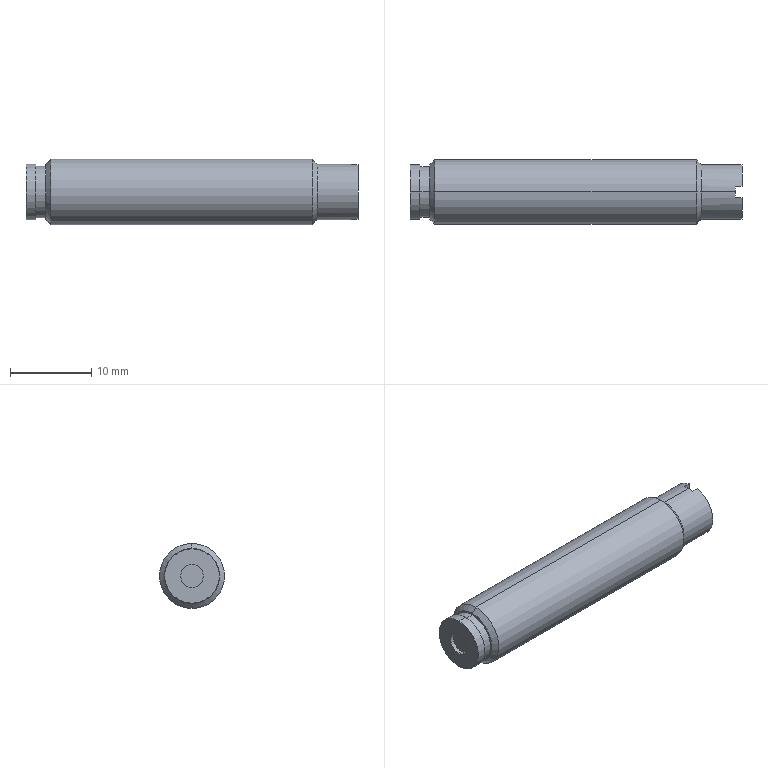Part | SolidWorks | features BaseBody 1 | 1 solid | 26 faces | box 40.8 x 8 x 8 mm | volume 1922 mm3 | cylinder 10 | plane 10 | cone 4 | torus 2 | commonest cylinder face diameters 6.8 x4 2.8 x2 6.3 x2 8 x2
STEP:
#1=CARTESIAN_POINT('',(0.5,0.,1.4));
#2=VERTEX_POINT('',#1);
#3=CARTESIAN_POINT('',(0.5,0.,-1.4));
#4=VERTEX_POINT('',#3);
#5=CARTESIAN_POINT('',(0.5,0.,0.));
#6=DIRECTION('',(1.,0.,0.));
#7=DIRECTION('',(0.,0.,-1.));
#8=AXIS2_PLACEMENT_3D('',#5,#6,#7);
#9=CIRCLE('',#8,1.4);
#10=EDGE_CURVE('',#2,#4,#9,.T.);
#11=ORIENTED_EDGE('',*,*,#10,.T.);
#12=CARTESIAN_POINT('',(0.,0.,-1.4));
#13=VERTEX_POINT('',#12);
#14=CARTESIAN_POINT('',(0.5,0.,-1.4));
#15=DIRECTION('',(-1.,0.,0.));
#16=VECTOR('',#15,1000.);
#17=LINE('',#14,#16);
#18=EDGE_CURVE('',#4,#13,#17,.T.);
#19=ORIENTED_EDGE('',*,*,#18,.T.);
#20=CARTESIAN_POINT('',(0.,0.,1.4));
#21=VERTEX_POINT('',#20);
#22=CARTESIAN_POINT('',(0.,0.,0.));
#23=DIRECTION('',(1.,0.,0.));
#24=DIRECTION('',(0.,0.,-1.));
#25=AXIS2_PLACEMENT_3D('',#22,#23,#24);
#26=CIRCLE('',#25,1.4);
#27=EDGE_CURVE('',#21,#13,#26,.T.);
#28=ORIENTED_EDGE('',*,*,#27,.F.);
#29=CARTESIAN_POINT('',(0.5,0.,1.4));
#30=DIRECTION('',(-1.,0.,0.));
#31=VECTOR('',#30,1000.);
#32=LINE('',#29,#31);
#33=EDGE_CURVE('',#2,#21,#32,.T.);
#34=ORIENTED_EDGE('',*,*,#33,.F.);
#35=EDGE_LOOP('',(#11,#19,#28,#34));
#36=FACE_OUTER_BOUND('',#35,.T.);
#37=CARTESIAN_POINT('',(0.5,0.,0.));
#38=DIRECTION('',(-1.,0.,0.));
#39=DIRECTION('',(0.,0.,1.));
#40=AXIS2_PLACEMENT_3D('',#37,#38,#39);
#41=CYLINDRICAL_SURFACE('',#40,1.4);
#42=ADVANCED_FACE('',(#36),#41,.F.);
#43=CARTESIAN_POINT('',(0.,0.,-3.35));
#44=VERTEX_POINT('',#43);
#45=CARTESIAN_POINT('',(0.,0.,3.35));
#46=VERTEX_POINT('',#45);
#47=CARTESIAN_POINT('',(0.,0.,0.));
#48=DIRECTION('',(1.,0.,0.));
#49=DIRECTION('',(0.,0.,-1.));
#50=AXIS2_PLACEMENT_3D('',#47,#48,#49);
#51=CIRCLE('',#50,3.35);
#52=EDGE_CURVE('',#44,#46,#51,.T.);
#53=ORIENTED_EDGE('',*,*,#52,.T.);
#54=CARTESIAN_POINT('',(0.05,0.,3.4));
#55=VERTEX_POINT('',#54);
#56=CARTESIAN_POINT('',(0.05,0.,3.35));
#57=DIRECTION('',(0.,1.,0.));
#58=DIRECTION('',(0.,0.,1.));
#59=AXIS2_PLACEMENT_3D('',#56,#57,#58);
#60=CIRCLE('',#59,0.05);
#61=EDGE_CURVE('',#46,#55,#60,.T.);
#62=ORIENTED_EDGE('',*,*,#61,.T.);
#63=CARTESIAN_POINT('',(0.05,0.,-3.4));
#64=VERTEX_POINT('',#63);
#65=CARTESIAN_POINT('',(0.05,0.,0.));
#66=DIRECTION('',(1.,0.,0.));
#67=DIRECTION('',(0.,0.,-1.));
#68=AXIS2_PLACEMENT_3D('',#65,#66,#67);
#69=CIRCLE('',#68,3.4);
#70=EDGE_CURVE('',#64,#55,#69,.T.);
#71=ORIENTED_EDGE('',*,*,#70,.F.);
#72=CARTESIAN_POINT('',(0.05,0.,-3.35));
#73=DIRECTION('',(0.,-1.,0.));
#74=DIRECTION('',(0.,0.,-1.));
#75=AXIS2_PLACEMENT_3D('',#72,#73,#74);
#76=CIRCLE('',#75,0.05);
#77=EDGE_CURVE('',#44,#64,#76,.T.);
#78=ORIENTED_EDGE('',*,*,#77,.F.);
#79=EDGE_LOOP('',(#53,#62,#71,#78));
#80=FACE_OUTER_BOUND('',#79,.T.);
#81=CARTESIAN_POINT('',(0.05,0.,0.));
#82=DIRECTION('',(1.,0.,0.));
#83=DIRECTION('',(0.,0.,-1.));
#84=AXIS2_PLACEMENT_3D('',#81,#82,#83);
#85=TOROIDAL_SURFACE('',#84,3.35,0.05);
#86=ADVANCED_FACE('',(#80),#85,.T.);
#87=ORIENTED_EDGE('',*,*,#70,.T.);
#88=CARTESIAN_POINT('',(1.2,0.,3.4));
#89=VERTEX_POINT('',#88);
#90=CARTESIAN_POINT('',(40.8,0.,3.4));
#91=DIRECTION('',(1.,0.,0.));
#92=VECTOR('',#91,1000.);
#93=LINE('',#90,#92);
#94=EDGE_CURVE('',#55,#89,#93,.T.);
#95=ORIENTED_EDGE('',*,*,#94,.T.);
#96=CARTESIAN_POINT('',(1.2,0.,-3.4));
#97=VERTEX_POINT('',#96);
#98=CARTESIAN_POINT('',(1.2,0.,0.));
#99=DIRECTION('',(1.,0.,0.));
#100=DIRECTION('',(0.,0.,-1.));
#101=AXIS2_PLACEMENT_3D('',#98,#99,#100);
#102=CIRCLE('',#101,3.4);
#103=EDGE_CURVE('',#97,#89,#102,.T.);
#104=ORIENTED_EDGE('',*,*,#103,.F.);
#105=CARTESIAN_POINT('',(40.8,0.,-3.4));
#106=DIRECTION('',(1.,0.,0.));
#107=VECTOR('',#106,1000.);
#108=LINE('',#105,#107);
#109=EDGE_CURVE('',#64,#97,#108,.T.);
#110=ORIENTED_EDGE('',*,*,#109,.F.);
#111=EDGE_LOOP('',(#87,#95,#104,#110));
#112=FACE_OUTER_BOUND('',#111,.T.);
#113=CARTESIAN_POINT('',(40.8,0.,0.));
#114=DIRECTION('',(1.,0.,0.));
#115=DIRECTION('',(0.,0.,-1.));
#116=AXIS2_PLACEMENT_3D('',#113,#114,#115);
#117=CYLINDRICAL_SURFACE('',#116,3.4);
#118=ADVANCED_FACE('',(#112),#117,.T.);
#119=CARTESIAN_POINT('',(1.2,0.,-3.15));
#120=VERTEX_POINT('',#119);
#121=CARTESIAN_POINT('',(1.2,0.,3.15));
#122=VERTEX_POINT('',#121);
#123=CARTESIAN_POINT('',(1.2,0.,0.));
#124=DIRECTION('',(1.,0.,0.));
#125=DIRECTION('',(0.,0.,-1.));
#126=AXIS2_PLACEMENT_3D('',#123,#124,#125);
#127=CIRCLE('',#126,3.15);
#128=EDGE_CURVE('',#120,#122,#127,.T.);
#129=ORIENTED_EDGE('',*,*,#128,.T.);
#130=CARTESIAN_POINT('',(2.4,0.,3.15));
#131=VERTEX_POINT('',#130);
#132=CARTESIAN_POINT('',(40.8,0.,3.15));
#133=DIRECTION('',(1.,0.,0.));
#134=VECTOR('',#133,1000.);
#135=LINE('',#132,#134);
#136=EDGE_CURVE('',#122,#131,#135,.T.);
#137=ORIENTED_EDGE('',*,*,#136,.T.);
#138=CARTESIAN_POINT('',(2.4,0.,-3.15));
#139=VERTEX_POINT('',#138);
#140=CARTESIAN_POINT('',(2.4,0.,0.));
#141=DIRECTION('',(1.,0.,0.));
#142=DIRECTION('',(0.,0.,-1.));
#143=AXIS2_PLACEMENT_3D('',#140,#141,#142);
#144=CIRCLE('',#143,3.15);
#145=EDGE_CURVE('',#139,#131,#144,.T.);
#146=ORIENTED_EDGE('',*,*,#145,.F.);
#147=CARTESIAN_POINT('',(40.8,0.,-3.15));
#148=DIRECTION('',(1.,0.,0.));
#149=VECTOR('',#148,1000.);
#150=LINE('',#147,#149);
#151=EDGE_CURVE('',#120,#139,#150,.T.);
#152=ORIENTED_EDGE('',*,*,#151,.F.);
#153=EDGE_LOOP('',(#129,#137,#146,#152));
#154=FACE_OUTER_BOUND('',#153,.T.);
#155=CARTESIAN_POINT('',(40.8,0.,0.));
#156=DIRECTION('',(1.,0.,0.));
#157=DIRECTION('',(0.,0.,-1.));
#158=AXIS2_PLACEMENT_3D('',#155,#156,#157);
#159=CYLINDRICAL_SURFACE('',#158,3.15);
#160=ADVANCED_FACE('',(#154),#159,.T.);
#161=CARTESIAN_POINT('',(2.4,0.,-3.387));
#162=VERTEX_POINT('',#161);
#163=CARTESIAN_POINT('',(2.4,0.,3.387));
#164=VERTEX_POINT('',#163);
#165=CARTESIAN_POINT('',(2.4,0.,0.));
#166=DIRECTION('',(1.,0.,0.));
#167=DIRECTION('',(0.,0.,-1.));
#168=AXIS2_PLACEMENT_3D('',#165,#166,#167);
#169=CIRCLE('',#168,3.387);
#170=EDGE_CURVE('',#162,#164,#169,.T.);
#171=ORIENTED_EDGE('',*,*,#170,.T.);
#172=CARTESIAN_POINT('',(3.014,0.,4.));
#173=VERTEX_POINT('',#172);
#174=CARTESIAN_POINT('',(2.4,0.,3.387));
#175=DIRECTION('',(0.7071,0.,0.7071));
#176=VECTOR('',#175,1000.);
#177=LINE('',#174,#176);
#178=EDGE_CURVE('',#164,#173,#177,.T.);
#179=ORIENTED_EDGE('',*,*,#178,.T.);
#180=CARTESIAN_POINT('',(3.014,0.,-4.));
#181=VERTEX_POINT('',#180);
#182=CARTESIAN_POINT('',(3.014,0.,0.));
#183=DIRECTION('',(1.,0.,0.));
#184=DIRECTION('',(0.,0.,-1.));
#185=AXIS2_PLACEMENT_3D('',#182,#183,#184);
#186=CIRCLE('',#185,4.);
#187=EDGE_CURVE('',#181,#173,#186,.T.);
#188=ORIENTED_EDGE('',*,*,#187,.F.);
#189=CARTESIAN_POINT('',(2.4,0.,-3.387));
#190=DIRECTION('',(0.7071,0.,-0.7071));
#191=VECTOR('',#190,1000.);
#192=LINE('',#189,#191);
#193=EDGE_CURVE('',#162,#181,#192,.T.);
#194=ORIENTED_EDGE('',*,*,#193,.F.);
#195=EDGE_LOOP('',(#171,#179,#188,#194));
#196=FACE_OUTER_BOUND('',#195,.T.);
#197=CARTESIAN_POINT('',(2.4,0.,0.));
#198=DIRECTION('',(1.,0.,0.));
#199=DIRECTION('',(0.,0.,-1.));
#200=AXIS2_PLACEMENT_3D('',#197,#198,#199);
#201=CONICAL_SURFACE('',#200,3.387,0.7854);
#202=ADVANCED_FACE('',(#196),#201,.T.);
#203=ORIENTED_EDGE('',*,*,#187,.T.);
#204=CARTESIAN_POINT('',(35.187,0.,4.));
#205=VERTEX_POINT('',#204);
#206=CARTESIAN_POINT('',(40.8,0.,4.));
#207=DIRECTION('',(1.,0.,0.));
#208=VECTOR('',#207,1000.);
#209=LINE('',#206,#208);
#210=EDGE_CURVE('',#173,#205,#209,.T.);
#211=ORIENTED_EDGE('',*,*,#210,.T.);
#212=CARTESIAN_POINT('',(35.187,0.,-4.));
#213=VERTEX_POINT('',#212);
#214=CARTESIAN_POINT('',(35.187,0.,0.));
#215=DIRECTION('',(1.,0.,0.));
#216=DIRECTION('',(0.,0.,-1.));
#217=AXIS2_PLACEMENT_3D('',#214,#215,#216);
#218=CIRCLE('',#217,4.);
#219=EDGE_CURVE('',#213,#205,#218,.T.);
#220=ORIENTED_EDGE('',*,*,#219,.F.);
#221=CARTESIAN_POINT('',(40.8,0.,-4.));
#222=DIRECTION('',(1.,0.,0.));
#223=VECTOR('',#222,1000.);
#224=LINE('',#221,#223);
#225=EDGE_CURVE('',#181,#213,#224,.T.);
#226=ORIENTED_EDGE('',*,*,#225,.F.);
#227=EDGE_LOOP('',(#203,#211,#220,#226));
#228=FACE_OUTER_BOUND('',#227,.T.);
#229=CARTESIAN_POINT('',(40.8,0.,0.));
#230=DIRECTION('',(1.,0.,0.));
#231=DIRECTION('',(0.,0.,-1.));
#232=AXIS2_PLACEMENT_3D('',#229,#230,#231);
#233=CYLINDRICAL_SURFACE('',#232,4.);
#234=ADVANCED_FACE('',(#228),#233,.T.);
#235=CARTESIAN_POINT('',(35.8,0.,-3.387));
#236=VERTEX_POINT('',#235);
#237=CARTESIAN_POINT('',(35.8,0.,3.387));
#238=VERTEX_POINT('',#237);
#239=CARTESIAN_POINT('',(35.8,0.,0.));
#240=DIRECTION('',(1.,0.,0.));
#241=DIRECTION('',(0.,0.,-1.));
#242=AXIS2_PLACEMENT_3D('',#239,#240,#241);
#243=CIRCLE('',#242,3.387);
#244=EDGE_CURVE('',#236,#238,#243,.T.);
#245=ORIENTED_EDGE('',*,*,#244,.F.);
#246=CARTESIAN_POINT('',(35.187,0.,-4.));
#247=DIRECTION('',(-0.7071,0.,-0.7071));
#248=VECTOR('',#247,1000.);
#249=LINE('',#246,#248);
#250=EDGE_CURVE('',#236,#213,#249,.T.);
#251=ORIENTED_EDGE('',*,*,#250,.T.);
#252=ORIENTED_EDGE('',*,*,#219,.T.);
#253=CARTESIAN_POINT('',(35.187,0.,4.));
#254=DIRECTION('',(-0.7071,0.,0.7071));
#255=VECTOR('',#254,1000.);
#256=LINE('',#253,#255);
#257=EDGE_CURVE('',#238,#205,#256,.T.);
#258=ORIENTED_EDGE('',*,*,#257,.F.);
#259=EDGE_LOOP('',(#245,#251,#252,#258));
#260=FACE_OUTER_BOUND('',#259,.T.);
#261=CARTESIAN_POINT('',(35.187,0.,0.));
#262=DIRECTION('',(-1.,0.,0.));
#263=DIRECTION('',(0.,0.,1.));
#264=AXIS2_PLACEMENT_3D('',#261,#262,#263);
#265=CONICAL_SURFACE('',#264,4.,0.7854);
#266=ADVANCED_FACE('',(#260),#265,.T.);
#267=CARTESIAN_POINT('',(35.8,0.,-3.4));
#268=VERTEX_POINT('',#267);
#269=CARTESIAN_POINT('',(35.8,0.,3.4));
#270=VERTEX_POINT('',#269);
#271=CARTESIAN_POINT('',(35.8,0.,0.));
#272=DIRECTION('',(1.,0.,0.));
#273=DIRECTION('',(0.,0.,-1.));
#274=AXIS2_PLACEMENT_3D('',#271,#272,#273);
#275=CIRCLE('',#274,3.4);
#276=EDGE_CURVE('',#268,#270,#275,.T.);
#277=ORIENTED_EDGE('',*,*,#276,.T.);
#278=CARTESIAN_POINT('',(40.,0.,3.4));
#279=VERTEX_POINT('',#278);
#280=CARTESIAN_POINT('',(40.8,0.,3.4));
#281=DIRECTION('',(1.,0.,0.));
#282=VECTOR('',#281,1000.);
#283=LINE('',#280,#282);
#284=EDGE_CURVE('',#270,#279,#283,.T.);
#285=ORIENTED_EDGE('',*,*,#284,.T.);
#286=CARTESIAN_POINT('',(40.,0.7,3.327));
#287=VERTEX_POINT('',#286);
#288=CARTESIAN_POINT('',(40.,0.,0.));
#289=DIRECTION('',(1.,0.,0.));
#290=DIRECTION('',(0.,0.2059,0.9786));
#291=AXIS2_PLACEMENT_3D('',#288,#289,#290);
#292=CIRCLE('',#291,3.4);
#293=EDGE_CURVE('',#287,#279,#292,.T.);
#294=ORIENTED_EDGE('',*,*,#293,.F.);
#295=CARTESIAN_POINT('',(40.8,0.7,3.327));
#296=VERTEX_POINT('',#295);
#297=CARTESIAN_POINT('',(40.8,0.7,3.327));
#298=DIRECTION('',(-1.,0.,0.));
#299=VECTOR('',#298,1000.);
#300=LINE('',#297,#299);
#301=EDGE_CURVE('',#296,#287,#300,.T.);
#302=ORIENTED_EDGE('',*,*,#301,.F.);
#303=CARTESIAN_POINT('',(40.8,0.7,-3.327));
#304=VERTEX_POINT('',#303);
#305=CARTESIAN_POINT('',(40.8,0.,0.));
#306=DIRECTION('',(1.,0.,0.));
#307=DIRECTION('',(0.,0.2059,-0.9786));
#308=AXIS2_PLACEMENT_3D('',#305,#306,#307);
#309=CIRCLE('',#308,3.4);
#310=EDGE_CURVE('',#304,#296,#309,.T.);
#311=ORIENTED_EDGE('',*,*,#310,.F.);
#312=CARTESIAN_POINT('',(40.,0.7,-3.327));
#313=VERTEX_POINT('',#312);
#314=CARTESIAN_POINT('',(40.,0.7,-3.327));
#315=DIRECTION('',(1.,0.,0.));
#316=VECTOR('',#315,1000.);
#317=LINE('',#314,#316);
#318=EDGE_CURVE('',#313,#304,#317,.T.);
#319=ORIENTED_EDGE('',*,*,#318,.F.);
#320=CARTESIAN_POINT('',(40.,0.,-3.4));
#321=VERTEX_POINT('',#320);
#322=CARTESIAN_POINT('',(40.,0.,0.));
#323=DIRECTION('',(1.,0.,0.));
#324=DIRECTION('',(0.,-0.2059,-0.9786));
#325=AXIS2_PLACEMENT_3D('',#322,#323,#324);
#326=CIRCLE('',#325,3.4);
#327=EDGE_CURVE('',#321,#313,#326,.T.);
#328=ORIENTED_EDGE('',*,*,#327,.F.);
#329=CARTESIAN_POINT('',(40.8,0.,-3.4));
#330=DIRECTION('',(1.,0.,0.));
#331=VECTOR('',#330,1000.);
#332=LINE('',#329,#331);
#333=EDGE_CURVE('',#268,#321,#332,.T.);
#334=ORIENTED_EDGE('',*,*,#333,.F.);
#335=EDGE_LOOP('',(#277,#285,#294,#302,#311,#319,#328,#334));
#336=FACE_OUTER_BOUND('',#335,.T.);
#337=CARTESIAN_POINT('',(40.8,0.,0.));
#338=DIRECTION('',(1.,0.,0.));
#339=DIRECTION('',(0.,0.,-1.));
#340=AXIS2_PLACEMENT_3D('',#337,#338,#339);
#341=CYLINDRICAL_SURFACE('',#340,3.4);
#342=ADVANCED_FACE('',(#336),#341,.T.);
#343=ORIENTED_EDGE('',*,*,#284,.F.);
#344=CARTESIAN_POINT('',(35.8,0.,0.));
#345=DIRECTION('',(1.,0.,0.));
#346=DIRECTION('',(0.,0.,-1.));
#347=AXIS2_PLACEMENT_3D('',#344,#345,#346);
#348=CIRCLE('',#347,3.4);
#349=EDGE_CURVE('',#270,#268,#348,.T.);
#350=ORIENTED_EDGE('',*,*,#349,.T.);
#351=ORIENTED_EDGE('',*,*,#333,.T.);
#352=CARTESIAN_POINT('',(40.,-0.7,-3.327));
#353=VERTEX_POINT('',#352);
#354=CARTESIAN_POINT('',(40.,0.,0.));
#355=DIRECTION('',(1.,0.,0.));
#356=DIRECTION('',(0.,-0.2059,-0.9786));
#357=AXIS2_PLACEMENT_3D('',#354,#355,#356);
#358=CIRCLE('',#357,3.4);
#359=EDGE_CURVE('',#353,#321,#358,.T.);
#360=ORIENTED_EDGE('',*,*,#359,.F.);
#361=CARTESIAN_POINT('',(40.8,-0.7,-3.327));
#362=VERTEX_POINT('',#361);
#363=CARTESIAN_POINT('',(40.8,-0.7,-3.327));
#364=DIRECTION('',(-1.,0.,0.));
#365=VECTOR('',#364,1000.);
#366=LINE('',#363,#365);
#367=EDGE_CURVE('',#362,#353,#366,.T.);
#368=ORIENTED_EDGE('',*,*,#367,.F.);
#369=CARTESIAN_POINT('',(40.8,-0.7,3.327));
#370=VERTEX_POINT('',#369);
#371=CARTESIAN_POINT('',(40.8,0.,0.));
#372=DIRECTION('',(1.,0.,0.));
#373=DIRECTION('',(0.,-0.2059,0.9786));
#374=AXIS2_PLACEMENT_3D('',#371,#372,#373);
#375=CIRCLE('',#374,3.4);
#376=EDGE_CURVE('',#370,#362,#375,.T.);
#377=ORIENTED_EDGE('',*,*,#376,.F.);
#378=CARTESIAN_POINT('',(40.,-0.7,3.327));
#379=VERTEX_POINT('',#378);
#380=CARTESIAN_POINT('',(40.,-0.7,3.327));
#381=DIRECTION('',(1.,0.,0.));
#382=VECTOR('',#381,1000.);
#383=LINE('',#380,#382);
#384=EDGE_CURVE('',#379,#370,#383,.T.);
#385=ORIENTED_EDGE('',*,*,#384,.F.);
#386=CARTESIAN_POINT('',(40.,0.,0.));
#387=DIRECTION('',(1.,0.,0.));
#388=DIRECTION('',(0.,0.2059,0.9786));
#389=AXIS2_PLACEMENT_3D('',#386,#387,#388);
#390=CIRCLE('',#389,3.4);
#391=EDGE_CURVE('',#279,#379,#390,.T.);
#392=ORIENTED_EDGE('',*,*,#391,.F.);
#393=EDGE_LOOP('',(#343,#350,#351,#360,#368,#377,#385,#392));
#394=FACE_OUTER_BOUND('',#393,.T.);
#395=CARTESIAN_POINT('',(40.8,0.,0.));
#396=DIRECTION('',(1.,0.,0.));
#397=DIRECTION('',(0.,0.,-1.));
#398=AXIS2_PLACEMENT_3D('',#395,#396,#397);
#399=CYLINDRICAL_SURFACE('',#398,3.4);
#400=ADVANCED_FACE('',(#394),#399,.T.);
#401=ORIENTED_EDGE('',*,*,#310,.T.);
#402=CARTESIAN_POINT('',(40.8,0.7,-3.327));
#403=DIRECTION('',(0.,0.,1.));
#404=VECTOR('',#403,1000.);
#405=LINE('',#402,#404);
#406=EDGE_CURVE('',#304,#296,#405,.T.);
#407=ORIENTED_EDGE('',*,*,#406,.F.);
#408=EDGE_LOOP('',(#401,#407));
#409=FACE_OUTER_BOUND('',#408,.T.);
#410=CARTESIAN_POINT('',(40.8,3.4,0.));
#411=DIRECTION('',(-1.,0.,0.));
#412=DIRECTION('',(0.,0.,1.));
#413=AXIS2_PLACEMENT_3D('',#410,#411,#412);
#414=PLANE('',#413);
#415=ADVANCED_FACE('',(#409),#414,.F.);
#416=ORIENTED_EDGE('',*,*,#318,.T.);
#417=ORIENTED_EDGE('',*,*,#406,.T.);
#418=ORIENTED_EDGE('',*,*,#301,.T.);
#419=CARTESIAN_POINT('',(40.,0.7,3.327));
#420=DIRECTION('',(0.,0.,-1.));
#421=VECTOR('',#420,1000.);
#422=LINE('',#419,#421);
#423=EDGE_CURVE('',#287,#313,#422,.T.);
#424=ORIENTED_EDGE('',*,*,#423,.T.);
#425=EDGE_LOOP('',(#416,#417,#418,#424));
#426=FACE_OUTER_BOUND('',#425,.T.);
#427=CARTESIAN_POINT('',(40.8,0.7,6.8));
#428=DIRECTION('',(0.,-1.,0.));
#429=DIRECTION('',(0.,0.,-1.));
#430=AXIS2_PLACEMENT_3D('',#427,#428,#429);
#431=PLANE('',#430);
#432=ADVANCED_FACE('',(#426),#431,.T.);
#433=ORIENTED_EDGE('',*,*,#293,.T.);
#434=ORIENTED_EDGE('',*,*,#391,.T.);
#435=CARTESIAN_POINT('',(40.,-0.7,3.327));
#436=DIRECTION('',(0.,0.,-1.));
#437=VECTOR('',#436,1000.);
#438=LINE('',#435,#437);
#439=EDGE_CURVE('',#379,#353,#438,.T.);
#440=ORIENTED_EDGE('',*,*,#439,.T.);
#441=ORIENTED_EDGE('',*,*,#359,.T.);
#442=ORIENTED_EDGE('',*,*,#327,.T.);
#443=ORIENTED_EDGE('',*,*,#423,.F.);
#444=EDGE_LOOP('',(#433,#434,#440,#441,#442,#443));
#445=FACE_OUTER_BOUND('',#444,.T.);
#446=CARTESIAN_POINT('',(40.,0.7,6.8));
#447=DIRECTION('',(1.,0.,0.));
#448=DIRECTION('',(0.,0.,-1.));
#449=AXIS2_PLACEMENT_3D('',#446,#447,#448);
#450=PLANE('',#449);
#451=ADVANCED_FACE('',(#445),#450,.T.);
#452=ORIENTED_EDGE('',*,*,#384,.T.);
#453=CARTESIAN_POINT('',(40.8,-0.7,3.327));
#454=DIRECTION('',(0.,0.,-1.));
#455=VECTOR('',#454,1000.);
#456=LINE('',#453,#455);
#457=EDGE_CURVE('',#370,#362,#456,.T.);
#458=ORIENTED_EDGE('',*,*,#457,.T.);
#459=ORIENTED_EDGE('',*,*,#367,.T.);
#460=ORIENTED_EDGE('',*,*,#439,.F.);
#461=EDGE_LOOP('',(#452,#458,#459,#460));
#462=FACE_OUTER_BOUND('',#461,.T.);
#463=CARTESIAN_POINT('',(40.,-0.7,6.8));
#464=DIRECTION('',(0.,1.,0.));
#465=DIRECTION('',(0.,0.,1.));
#466=AXIS2_PLACEMENT_3D('',#463,#464,#465);
#467=PLANE('',#466);
#468=ADVANCED_FACE('',(#462),#467,.T.);
#469=ORIENTED_EDGE('',*,*,#457,.F.);
#470=ORIENTED_EDGE('',*,*,#376,.T.);
#471=EDGE_LOOP('',(#469,#470));
#472=FACE_OUTER_BOUND('',#471,.T.);
#473=CARTESIAN_POINT('',(40.8,3.4,0.));
#474=DIRECTION('',(-1.,0.,0.));
#475=DIRECTION('',(0.,0.,1.));
#476=AXIS2_PLACEMENT_3D('',#473,#474,#475);
#477=PLANE('',#476);
#478=ADVANCED_FACE('',(#472),#477,.F.);
#479=ORIENTED_EDGE('',*,*,#276,.F.);
#480=ORIENTED_EDGE('',*,*,#349,.F.);
#481=EDGE_LOOP('',(#479,#480));
#482=FACE_OUTER_BOUND('',#481,.T.);
#483=CARTESIAN_POINT('',(35.8,0.,0.));
#484=DIRECTION('',(1.,0.,0.));
#485=DIRECTION('',(0.,0.,-1.));
#486=AXIS2_PLACEMENT_3D('',#483,#484,#485);
#487=CIRCLE('',#486,3.387);
#488=EDGE_CURVE('',#238,#236,#487,.T.);
#489=ORIENTED_EDGE('',*,*,#488,.T.);
#490=ORIENTED_EDGE('',*,*,#244,.T.);
#491=EDGE_LOOP('',(#489,#490));
#492=FACE_BOUND('',#491,.T.);
#493=CARTESIAN_POINT('',(35.8,3.387,0.));
#494=DIRECTION('',(1.,0.,0.));
#495=DIRECTION('',(0.,0.,-1.));
#496=AXIS2_PLACEMENT_3D('',#493,#494,#495);
#497=PLANE('',#496);
#498=ADVANCED_FACE('',(#482,#492),#497,.F.);
#499=ORIENTED_EDGE('',*,*,#250,.F.);
#500=ORIENTED_EDGE('',*,*,#488,.F.);
#501=ORIENTED_EDGE('',*,*,#257,.T.);
#502=CARTESIAN_POINT('',(35.187,0.,0.));
#503=DIRECTION('',(1.,0.,0.));
#504=DIRECTION('',(0.,0.,-1.));
#505=AXIS2_PLACEMENT_3D('',#502,#503,#504);
#506=CIRCLE('',#505,4.);
#507=EDGE_CURVE('',#205,#213,#506,.T.);
#508=ORIENTED_EDGE('',*,*,#507,.T.);
#509=EDGE_LOOP('',(#499,#500,#501,#508));
#510=FACE_OUTER_BOUND('',#509,.T.);
#511=CARTESIAN_POINT('',(35.187,0.,0.));
#512=DIRECTION('',(-1.,0.,0.));
#513=DIRECTION('',(0.,0.,1.));
#514=AXIS2_PLACEMENT_3D('',#511,#512,#513);
#515=CONICAL_SURFACE('',#514,4.,0.7854);
#516=ADVANCED_FACE('',(#510),#515,.T.);
#517=ORIENTED_EDGE('',*,*,#210,.F.);
#518=CARTESIAN_POINT('',(3.014,0.,0.));
#519=DIRECTION('',(1.,0.,0.));
#520=DIRECTION('',(0.,0.,-1.));
#521=AXIS2_PLACEMENT_3D('',#518,#519,#520);
#522=CIRCLE('',#521,4.);
#523=EDGE_CURVE('',#173,#181,#522,.T.);
#524=ORIENTED_EDGE('',*,*,#523,.T.);
#525=ORIENTED_EDGE('',*,*,#225,.T.);
#526=ORIENTED_EDGE('',*,*,#507,.F.);
#527=EDGE_LOOP('',(#517,#524,#525,#526));
#528=FACE_OUTER_BOUND('',#527,.T.);
#529=CARTESIAN_POINT('',(40.8,0.,0.));
#530=DIRECTION('',(1.,0.,0.));
#531=DIRECTION('',(0.,0.,-1.));
#532=AXIS2_PLACEMENT_3D('',#529,#530,#531);
#533=CYLINDRICAL_SURFACE('',#532,4.);
#534=ADVANCED_FACE('',(#528),#533,.T.);
#535=ORIENTED_EDGE('',*,*,#178,.F.);
#536=CARTESIAN_POINT('',(2.4,0.,0.));
#537=DIRECTION('',(1.,0.,0.));
#538=DIRECTION('',(0.,0.,-1.));
#539=AXIS2_PLACEMENT_3D('',#536,#537,#538);
#540=CIRCLE('',#539,3.387);
#541=EDGE_CURVE('',#164,#162,#540,.T.);
#542=ORIENTED_EDGE('',*,*,#541,.T.);
#543=ORIENTED_EDGE('',*,*,#193,.T.);
#544=ORIENTED_EDGE('',*,*,#523,.F.);
#545=EDGE_LOOP('',(#535,#542,#543,#544));
#546=FACE_OUTER_BOUND('',#545,.T.);
#547=CARTESIAN_POINT('',(2.4,0.,0.));
#548=DIRECTION('',(1.,0.,0.));
#549=DIRECTION('',(0.,0.,-1.));
#550=AXIS2_PLACEMENT_3D('',#547,#548,#549);
#551=CONICAL_SURFACE('',#550,3.387,0.7854);
#552=ADVANCED_FACE('',(#546),#551,.T.);
#553=ORIENTED_EDGE('',*,*,#170,.F.);
#554=ORIENTED_EDGE('',*,*,#541,.F.);
#555=EDGE_LOOP('',(#553,#554));
#556=FACE_OUTER_BOUND('',#555,.T.);
#557=ORIENTED_EDGE('',*,*,#145,.T.);
#558=CARTESIAN_POINT('',(2.4,0.,0.));
#559=DIRECTION('',(1.,0.,0.));
#560=DIRECTION('',(0.,0.,-1.));
#561=AXIS2_PLACEMENT_3D('',#558,#559,#560);
#562=CIRCLE('',#561,3.15);
#563=EDGE_CURVE('',#131,#139,#562,.T.);
#564=ORIENTED_EDGE('',*,*,#563,.T.);
#565=EDGE_LOOP('',(#557,#564));
#566=FACE_BOUND('',#565,.T.);
#567=CARTESIAN_POINT('',(2.4,3.15,0.));
#568=DIRECTION('',(1.,0.,0.));
#569=DIRECTION('',(0.,0.,-1.));
#570=AXIS2_PLACEMENT_3D('',#567,#568,#569);
#571=PLANE('',#570);
#572=ADVANCED_FACE('',(#556,#566),#571,.F.);
#573=ORIENTED_EDGE('',*,*,#136,.F.);
#574=CARTESIAN_POINT('',(1.2,0.,0.));
#575=DIRECTION('',(1.,0.,0.));
#576=DIRECTION('',(0.,0.,-1.));
#577=AXIS2_PLACEMENT_3D('',#574,#575,#576);
#578=CIRCLE('',#577,3.15);
#579=EDGE_CURVE('',#122,#120,#578,.T.);
#580=ORIENTED_EDGE('',*,*,#579,.T.);
#581=ORIENTED_EDGE('',*,*,#151,.T.);
#582=ORIENTED_EDGE('',*,*,#563,.F.);
#583=EDGE_LOOP('',(#573,#580,#581,#582));
#584=FACE_OUTER_BOUND('',#583,.T.);
#585=CARTESIAN_POINT('',(40.8,0.,0.));
#586=DIRECTION('',(1.,0.,0.));
#587=DIRECTION('',(0.,0.,-1.));
#588=AXIS2_PLACEMENT_3D('',#585,#586,#587);
#589=CYLINDRICAL_SURFACE('',#588,3.15);
#590=ADVANCED_FACE('',(#584),#589,.T.);
#591=ORIENTED_EDGE('',*,*,#128,.F.);
#592=ORIENTED_EDGE('',*,*,#579,.F.);
#593=EDGE_LOOP('',(#591,#592));
#594=FACE_BOUND('',#593,.T.);
#595=ORIENTED_EDGE('',*,*,#103,.T.);
#596=CARTESIAN_POINT('',(1.2,0.,0.));
#597=DIRECTION('',(1.,0.,0.));
#598=DIRECTION('',(0.,0.,-1.));
#599=AXIS2_PLACEMENT_3D('',#596,#597,#598);
#600=CIRCLE('',#599,3.4);
#601=EDGE_CURVE('',#89,#97,#600,.T.);
#602=ORIENTED_EDGE('',*,*,#601,.T.);
#603=EDGE_LOOP('',(#595,#602));
#604=FACE_OUTER_BOUND('',#603,.T.);
#605=CARTESIAN_POINT('',(1.2,3.4,0.));
#606=DIRECTION('',(-1.,0.,0.));
#607=DIRECTION('',(0.,0.,1.));
#608=AXIS2_PLACEMENT_3D('',#605,#606,#607);
#609=PLANE('',#608);
#610=ADVANCED_FACE('',(#594,#604),#609,.F.);
#611=ORIENTED_EDGE('',*,*,#94,.F.);
#612=CARTESIAN_POINT('',(0.05,0.,0.));
#613=DIRECTION('',(1.,0.,0.));
#614=DIRECTION('',(0.,0.,-1.));
#615=AXIS2_PLACEMENT_3D('',#612,#613,#614);
#616=CIRCLE('',#615,3.4);
#617=EDGE_CURVE('',#55,#64,#616,.T.);
#618=ORIENTED_EDGE('',*,*,#617,.T.);
#619=ORIENTED_EDGE('',*,*,#109,.T.);
#620=ORIENTED_EDGE('',*,*,#601,.F.);
#621=EDGE_LOOP('',(#611,#618,#619,#620));
#622=FACE_OUTER_BOUND('',#621,.T.);
#623=CARTESIAN_POINT('',(40.8,0.,0.));
#624=DIRECTION('',(1.,0.,0.));
#625=DIRECTION('',(0.,0.,-1.));
#626=AXIS2_PLACEMENT_3D('',#623,#624,#625);
#627=CYLINDRICAL_SURFACE('',#626,3.4);
#628=ADVANCED_FACE('',(#622),#627,.T.);
#629=ORIENTED_EDGE('',*,*,#61,.F.);
#630=CARTESIAN_POINT('',(0.,0.,0.));
#631=DIRECTION('',(1.,0.,0.));
#632=DIRECTION('',(0.,0.,-1.));
#633=AXIS2_PLACEMENT_3D('',#630,#631,#632);
#634=CIRCLE('',#633,3.35);
#635=EDGE_CURVE('',#46,#44,#634,.T.);
#636=ORIENTED_EDGE('',*,*,#635,.T.);
#637=ORIENTED_EDGE('',*,*,#77,.T.);
#638=ORIENTED_EDGE('',*,*,#617,.F.);
#639=EDGE_LOOP('',(#629,#636,#637,#638));
#640=FACE_OUTER_BOUND('',#639,.T.);
#641=CARTESIAN_POINT('',(0.05,0.,0.));
#642=DIRECTION('',(1.,0.,0.));
#643=DIRECTION('',(0.,0.,-1.));
#644=AXIS2_PLACEMENT_3D('',#641,#642,#643);
#645=TOROIDAL_SURFACE('',#644,3.35,0.05);
#646=ADVANCED_FACE('',(#640),#645,.T.);
#647=ORIENTED_EDGE('',*,*,#52,.F.);
#648=ORIENTED_EDGE('',*,*,#635,.F.);
#649=EDGE_LOOP('',(#647,#648));
#650=FACE_OUTER_BOUND('',#649,.T.);
#651=ORIENTED_EDGE('',*,*,#27,.T.);
#652=CARTESIAN_POINT('',(0.,0.,0.));
#653=DIRECTION('',(1.,0.,0.));
#654=DIRECTION('',(0.,0.,-1.));
#655=AXIS2_PLACEMENT_3D('',#652,#653,#654);
#656=CIRCLE('',#655,1.4);
#657=EDGE_CURVE('',#13,#21,#656,.T.);
#658=ORIENTED_EDGE('',*,*,#657,.T.);
#659=EDGE_LOOP('',(#651,#658));
#660=FACE_BOUND('',#659,.T.);
#661=CARTESIAN_POINT('',(0.,0.,0.));
#662=DIRECTION('',(1.,0.,0.));
#663=DIRECTION('',(0.,0.,-1.));
#664=AXIS2_PLACEMENT_3D('',#661,#662,#663);
#665=PLANE('',#664);
#666=ADVANCED_FACE('',(#650,#660),#665,.F.);
#667=ORIENTED_EDGE('',*,*,#18,.F.);
#668=CARTESIAN_POINT('',(0.5,0.,0.));
#669=DIRECTION('',(1.,0.,0.));
#670=DIRECTION('',(0.,0.,-1.));
#671=AXIS2_PLACEMENT_3D('',#668,#669,#670);
#672=CIRCLE('',#671,1.4);
#673=EDGE_CURVE('',#4,#2,#672,.T.);
#674=ORIENTED_EDGE('',*,*,#673,.T.);
#675=ORIENTED_EDGE('',*,*,#33,.T.);
#676=ORIENTED_EDGE('',*,*,#657,.F.);
#677=EDGE_LOOP('',(#667,#674,#675,#676));
#678=FACE_OUTER_BOUND('',#677,.T.);
#679=CARTESIAN_POINT('',(0.5,0.,0.));
#680=DIRECTION('',(-1.,0.,0.));
#681=DIRECTION('',(0.,0.,1.));
#682=AXIS2_PLACEMENT_3D('',#679,#680,#681);
#683=CYLINDRICAL_SURFACE('',#682,1.4);
#684=ADVANCED_FACE('',(#678),#683,.F.);
#685=ORIENTED_EDGE('',*,*,#10,.F.);
#686=ORIENTED_EDGE('',*,*,#673,.F.);
#687=EDGE_LOOP('',(#685,#686));
#688=FACE_OUTER_BOUND('',#687,.T.);
#689=CARTESIAN_POINT('',(0.5,0.,0.));
#690=DIRECTION('',(1.,0.,0.));
#691=DIRECTION('',(0.,0.,-1.));
#692=AXIS2_PLACEMENT_3D('',#689,#690,#691);
#693=PLANE('',#692);
#694=ADVANCED_FACE('',(#688),#693,.F.);
#695=CLOSED_SHELL('',(#42,#86,#118,#160,#202,#234,#266,#342,#400,#415,#432,#451,#468,#478,#498,#516,#534,#552,#572,#590,#610,#628,#646,#666,#684,#694));
#696=MANIFOLD_SOLID_BREP('',#695);
#697=CARTESIAN_POINT('',(0.,0.,0.));
#698=DIRECTION('',(0.,0.,1.));
#699=DIRECTION('',(1.,0.,0.));
#700=AXIS2_PLACEMENT_3D('',#697,#698,#699);
#701=(LENGTH_UNIT()NAMED_UNIT(*)SI_UNIT(.MILLI.,.METRE.));
#702=UNCERTAINTY_MEASURE_WITH_UNIT(LENGTH_MEASURE(0.00001),#701,'','');
#703=(NAMED_UNIT(*)PLANE_ANGLE_UNIT()SI_UNIT($,.RADIAN.));
#704=(NAMED_UNIT(*)SI_UNIT($,.STERADIAN.)SOLID_ANGLE_UNIT());
#705=(GEOMETRIC_REPRESENTATION_CONTEXT(3)GLOBAL_UNCERTAINTY_ASSIGNED_CONTEXT((#702))GLOBAL_UNIT_ASSIGNED_CONTEXT((#701,#703,#704))REPRESENTATION_CONTEXT('',''));
#706=ADVANCED_BREP_SHAPE_REPRESENTATION('',(#696,#700),#705);